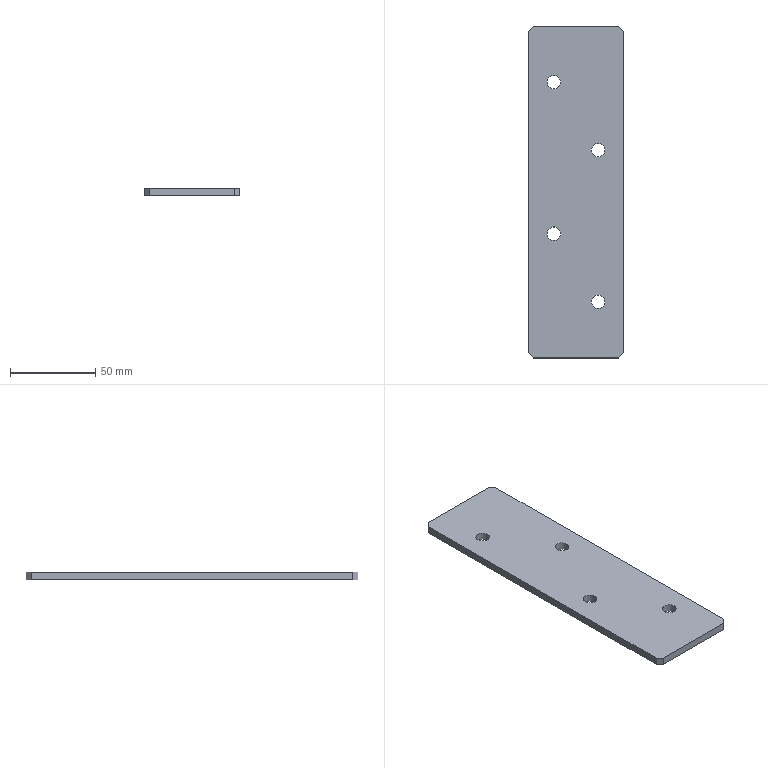Part | STEP file | 1_id70_x_t | 1 solid | 14 faces | box 56 x 195 x 4.5 mm | volume 48168 mm3 | plane 10 | cylinder 4 | commonest cylinder face diameters 7.938 x4
STEP:
#1=CARTESIAN_POINT('',(0.,0.,0.));
#2=DIRECTION('',(0.,0.,1.));
#3=DIRECTION('',(1.,0.,0.));
#4=AXIS2_PLACEMENT_3D('',#1,#2,#3);
#5=CARTESIAN_POINT('',(489.325,80.,86.035));
#6=VERTEX_POINT('',#5);
#7=CARTESIAN_POINT('',(489.325,80.,90.535));
#8=VERTEX_POINT('',#7);
#9=CARTESIAN_POINT('',(489.325,80.,86.035));
#10=DIRECTION('',(0.,0.,1.));
#11=VECTOR('',#10,1.);
#12=LINE('',#9,#11);
#13=CARTESIAN_POINT('',(489.325,80.,86.035));
#14=DIRECTION('',(0.7071,-0.7071,0.));
#15=DIRECTION('',(0.7071,0.7071,0.));
#16=AXIS2_PLACEMENT_3D('',#13,#14,#15);
#17=PLANE('',#16);
#18=CARTESIAN_POINT('',(0.,0.));
#19=DIRECTION('',(0.,1.));
#20=VECTOR('',#19,1.);
#21=LINE('',#18,#20);
#22=(GEOMETRIC_REPRESENTATION_CONTEXT(2)PARAMETRIC_REPRESENTATION_CONTEXT()REPRESENTATION_CONTEXT('',''));
#23=DEFINITIONAL_REPRESENTATION('',(#21),#22);
#24=PCURVE('',#17,#23);
#25=CARTESIAN_POINT('',(491.788,80.,86.035));
#26=DIRECTION('',(0.,-1.,0.));
#27=DIRECTION('',(1.,0.,0.));
#28=AXIS2_PLACEMENT_3D('',#25,#26,#27);
#29=PLANE('',#28);
#30=CARTESIAN_POINT('',(-2.463,0.));
#31=DIRECTION('',(0.,1.));
#32=VECTOR('',#31,1.);
#33=LINE('',#30,#32);
#34=(GEOMETRIC_REPRESENTATION_CONTEXT(2)PARAMETRIC_REPRESENTATION_CONTEXT()REPRESENTATION_CONTEXT('',''));
#35=DEFINITIONAL_REPRESENTATION('',(#33),#34);
#36=PCURVE('',#29,#35);
#37=SURFACE_CURVE('',#12,(#24,#36),.PCURVE_S1.);
#38=EDGE_CURVE('',#6,#8,#37,.T.);
#39=ORIENTED_EDGE('',*,*,#38,.F.);
#40=CARTESIAN_POINT('',(492.325,83.,86.035));
#41=VERTEX_POINT('',#40);
#42=CARTESIAN_POINT('',(489.325,80.,86.035));
#43=DIRECTION('',(0.7071,0.7071,0.));
#44=VECTOR('',#43,1.);
#45=LINE('',#42,#44);
#46=CARTESIAN_POINT('',(0.,0.));
#47=DIRECTION('',(1.,0.));
#48=VECTOR('',#47,1.);
#49=LINE('',#46,#48);
#50=(GEOMETRIC_REPRESENTATION_CONTEXT(2)PARAMETRIC_REPRESENTATION_CONTEXT()REPRESENTATION_CONTEXT('',''));
#51=DEFINITIONAL_REPRESENTATION('',(#49),#50);
#52=PCURVE('',#17,#51);
#53=CARTESIAN_POINT('',(491.788,255.,86.035));
#54=DIRECTION('',(0.,0.,1.));
#55=DIRECTION('',(1.,0.,0.));
#56=AXIS2_PLACEMENT_3D('',#53,#54,#55);
#57=PLANE('',#56);
#58=CARTESIAN_POINT('',(-2.463,-175.));
#59=DIRECTION('',(0.7071,0.7071));
#60=VECTOR('',#59,1.);
#61=LINE('',#58,#60);
#62=(GEOMETRIC_REPRESENTATION_CONTEXT(2)PARAMETRIC_REPRESENTATION_CONTEXT()REPRESENTATION_CONTEXT('',''));
#63=DEFINITIONAL_REPRESENTATION('',(#61),#62);
#64=PCURVE('',#57,#63);
#65=SURFACE_CURVE('',#45,(#52,#64),.PCURVE_S1.);
#66=EDGE_CURVE('',#6,#41,#65,.T.);
#67=ORIENTED_EDGE('',*,*,#66,.T.);
#68=CARTESIAN_POINT('',(492.325,83.,90.535));
#69=VERTEX_POINT('',#68);
#70=CARTESIAN_POINT('',(492.325,83.,86.035));
#71=DIRECTION('',(0.,0.,1.));
#72=VECTOR('',#71,1.);
#73=LINE('',#70,#72);
#74=CARTESIAN_POINT('',(4.243,0.));
#75=DIRECTION('',(0.,1.));
#76=VECTOR('',#75,1.);
#77=LINE('',#74,#76);
#78=(GEOMETRIC_REPRESENTATION_CONTEXT(2)PARAMETRIC_REPRESENTATION_CONTEXT()REPRESENTATION_CONTEXT('',''));
#79=DEFINITIONAL_REPRESENTATION('',(#77),#78);
#80=PCURVE('',#17,#79);
#81=CARTESIAN_POINT('',(492.325,255.,86.035));
#82=DIRECTION('',(1.,0.,0.));
#83=DIRECTION('',(0.,1.,0.));
#84=AXIS2_PLACEMENT_3D('',#81,#82,#83);
#85=PLANE('',#84);
#86=CARTESIAN_POINT('',(-172.,0.));
#87=DIRECTION('',(0.,1.));
#88=VECTOR('',#87,1.);
#89=LINE('',#86,#88);
#90=(GEOMETRIC_REPRESENTATION_CONTEXT(2)PARAMETRIC_REPRESENTATION_CONTEXT()REPRESENTATION_CONTEXT('',''));
#91=DEFINITIONAL_REPRESENTATION('',(#89),#90);
#92=PCURVE('',#85,#91);
#93=SURFACE_CURVE('',#73,(#80,#92),.PCURVE_S1.);
#94=EDGE_CURVE('',#41,#69,#93,.T.);
#95=ORIENTED_EDGE('',*,*,#94,.T.);
#96=CARTESIAN_POINT('',(489.325,80.,90.535));
#97=DIRECTION('',(0.7071,0.7071,0.));
#98=VECTOR('',#97,1.);
#99=LINE('',#96,#98);
#100=CARTESIAN_POINT('',(0.,4.5));
#101=DIRECTION('',(1.,0.));
#102=VECTOR('',#101,1.);
#103=LINE('',#100,#102);
#104=(GEOMETRIC_REPRESENTATION_CONTEXT(2)PARAMETRIC_REPRESENTATION_CONTEXT()REPRESENTATION_CONTEXT('',''));
#105=DEFINITIONAL_REPRESENTATION('',(#103),#104);
#106=PCURVE('',#17,#105);
#107=CARTESIAN_POINT('',(491.788,255.,90.535));
#108=DIRECTION('',(0.,0.,1.));
#109=DIRECTION('',(1.,0.,0.));
#110=AXIS2_PLACEMENT_3D('',#107,#108,#109);
#111=PLANE('',#110);
#112=CARTESIAN_POINT('',(-2.463,-175.));
#113=DIRECTION('',(0.7071,0.7071));
#114=VECTOR('',#113,1.);
#115=LINE('',#112,#114);
#116=(GEOMETRIC_REPRESENTATION_CONTEXT(2)PARAMETRIC_REPRESENTATION_CONTEXT()REPRESENTATION_CONTEXT('',''));
#117=DEFINITIONAL_REPRESENTATION('',(#115),#116);
#118=PCURVE('',#111,#117);
#119=SURFACE_CURVE('',#99,(#106,#118),.PCURVE_S1.);
#120=EDGE_CURVE('',#8,#69,#119,.T.);
#121=ORIENTED_EDGE('',*,*,#120,.F.);
#122=EDGE_LOOP('',(#39,#67,#95,#121));
#123=FACE_BOUND('',#122,.T.);
#124=ADVANCED_FACE('',(#123),#17,.T.);
#125=ORIENTED_EDGE('',*,*,#94,.F.);
#126=CARTESIAN_POINT('',(492.325,272.,86.035));
#127=VERTEX_POINT('',#126);
#128=CARTESIAN_POINT('',(492.325,255.,86.035));
#129=DIRECTION('',(0.,-1.,0.));
#130=VECTOR('',#129,1.);
#131=LINE('',#128,#130);
#132=CARTESIAN_POINT('',(0.,0.));
#133=DIRECTION('',(-1.,0.));
#134=VECTOR('',#133,1.);
#135=LINE('',#132,#134);
#136=(GEOMETRIC_REPRESENTATION_CONTEXT(2)PARAMETRIC_REPRESENTATION_CONTEXT()REPRESENTATION_CONTEXT('',''));
#137=DEFINITIONAL_REPRESENTATION('',(#135),#136);
#138=PCURVE('',#85,#137);
#139=CARTESIAN_POINT('',(0.5375,0.));
#140=DIRECTION('',(0.,-1.));
#141=VECTOR('',#140,1.);
#142=LINE('',#139,#141);
#143=(GEOMETRIC_REPRESENTATION_CONTEXT(2)PARAMETRIC_REPRESENTATION_CONTEXT()REPRESENTATION_CONTEXT('',''));
#144=DEFINITIONAL_REPRESENTATION('',(#142),#143);
#145=PCURVE('',#57,#144);
#146=SURFACE_CURVE('',#131,(#138,#145),.PCURVE_S1.);
#147=EDGE_CURVE('',#127,#41,#146,.T.);
#148=ORIENTED_EDGE('',*,*,#147,.F.);
#149=CARTESIAN_POINT('',(492.325,272.,90.535));
#150=VERTEX_POINT('',#149);
#151=CARTESIAN_POINT('',(492.325,272.,86.035));
#152=DIRECTION('',(0.,0.,1.));
#153=VECTOR('',#152,1.);
#154=LINE('',#151,#153);
#155=CARTESIAN_POINT('',(17.,0.));
#156=DIRECTION('',(0.,1.));
#157=VECTOR('',#156,1.);
#158=LINE('',#155,#157);
#159=(GEOMETRIC_REPRESENTATION_CONTEXT(2)PARAMETRIC_REPRESENTATION_CONTEXT()REPRESENTATION_CONTEXT('',''));
#160=DEFINITIONAL_REPRESENTATION('',(#158),#159);
#161=PCURVE('',#85,#160);
#162=CARTESIAN_POINT('',(492.325,272.,86.035));
#163=DIRECTION('',(0.7071,0.7071,0.));
#164=DIRECTION('',(-0.7071,0.7071,0.));
#165=AXIS2_PLACEMENT_3D('',#162,#163,#164);
#166=PLANE('',#165);
#167=CARTESIAN_POINT('',(0.,0.));
#168=DIRECTION('',(0.,1.));
#169=VECTOR('',#168,1.);
#170=LINE('',#167,#169);
#171=(GEOMETRIC_REPRESENTATION_CONTEXT(2)PARAMETRIC_REPRESENTATION_CONTEXT()REPRESENTATION_CONTEXT('',''));
#172=DEFINITIONAL_REPRESENTATION('',(#170),#171);
#173=PCURVE('',#166,#172);
#174=SURFACE_CURVE('',#154,(#161,#173),.PCURVE_S1.);
#175=EDGE_CURVE('',#127,#150,#174,.T.);
#176=ORIENTED_EDGE('',*,*,#175,.T.);
#177=CARTESIAN_POINT('',(492.325,255.,90.535));
#178=DIRECTION('',(0.,-1.,0.));
#179=VECTOR('',#178,1.);
#180=LINE('',#177,#179);
#181=CARTESIAN_POINT('',(0.,4.5));
#182=DIRECTION('',(-1.,0.));
#183=VECTOR('',#182,1.);
#184=LINE('',#181,#183);
#185=(GEOMETRIC_REPRESENTATION_CONTEXT(2)PARAMETRIC_REPRESENTATION_CONTEXT()REPRESENTATION_CONTEXT('',''));
#186=DEFINITIONAL_REPRESENTATION('',(#184),#185);
#187=PCURVE('',#85,#186);
#188=CARTESIAN_POINT('',(0.5375,0.));
#189=DIRECTION('',(0.,-1.));
#190=VECTOR('',#189,1.);
#191=LINE('',#188,#190);
#192=(GEOMETRIC_REPRESENTATION_CONTEXT(2)PARAMETRIC_REPRESENTATION_CONTEXT()REPRESENTATION_CONTEXT('',''));
#193=DEFINITIONAL_REPRESENTATION('',(#191),#192);
#194=PCURVE('',#111,#193);
#195=SURFACE_CURVE('',#180,(#187,#194),.PCURVE_S1.);
#196=EDGE_CURVE('',#150,#69,#195,.T.);
#197=ORIENTED_EDGE('',*,*,#196,.T.);
#198=EDGE_LOOP('',(#125,#148,#176,#197));
#199=FACE_BOUND('',#198,.T.);
#200=ADVANCED_FACE('',(#199),#85,.T.);
#201=ORIENTED_EDGE('',*,*,#175,.F.);
#202=CARTESIAN_POINT('',(489.325,275.,86.035));
#203=VERTEX_POINT('',#202);
#204=CARTESIAN_POINT('',(492.325,272.,86.035));
#205=DIRECTION('',(-0.7071,0.7071,0.));
#206=VECTOR('',#205,1.);
#207=LINE('',#204,#206);
#208=CARTESIAN_POINT('',(0.,0.));
#209=DIRECTION('',(1.,0.));
#210=VECTOR('',#209,1.);
#211=LINE('',#208,#210);
#212=(GEOMETRIC_REPRESENTATION_CONTEXT(2)PARAMETRIC_REPRESENTATION_CONTEXT()REPRESENTATION_CONTEXT('',''));
#213=DEFINITIONAL_REPRESENTATION('',(#211),#212);
#214=PCURVE('',#166,#213);
#215=CARTESIAN_POINT('',(0.5375,17.));
#216=DIRECTION('',(-0.7071,0.7071));
#217=VECTOR('',#216,1.);
#218=LINE('',#215,#217);
#219=(GEOMETRIC_REPRESENTATION_CONTEXT(2)PARAMETRIC_REPRESENTATION_CONTEXT()REPRESENTATION_CONTEXT('',''));
#220=DEFINITIONAL_REPRESENTATION('',(#218),#219);
#221=PCURVE('',#57,#220);
#222=SURFACE_CURVE('',#207,(#214,#221),.PCURVE_S1.);
#223=EDGE_CURVE('',#127,#203,#222,.T.);
#224=ORIENTED_EDGE('',*,*,#223,.T.);
#225=CARTESIAN_POINT('',(489.325,275.,90.535));
#226=VERTEX_POINT('',#225);
#227=CARTESIAN_POINT('',(489.325,275.,86.035));
#228=DIRECTION('',(0.,0.,1.));
#229=VECTOR('',#228,1.);
#230=LINE('',#227,#229);
#231=CARTESIAN_POINT('',(4.243,0.));
#232=DIRECTION('',(0.,1.));
#233=VECTOR('',#232,1.);
#234=LINE('',#231,#233);
#235=(GEOMETRIC_REPRESENTATION_CONTEXT(2)PARAMETRIC_REPRESENTATION_CONTEXT()REPRESENTATION_CONTEXT('',''));
#236=DEFINITIONAL_REPRESENTATION('',(#234),#235);
#237=PCURVE('',#166,#236);
#238=CARTESIAN_POINT('',(491.788,275.,86.035));
#239=DIRECTION('',(0.,-1.,0.));
#240=DIRECTION('',(1.,0.,0.));
#241=AXIS2_PLACEMENT_3D('',#238,#239,#240);
#242=PLANE('',#241);
#243=CARTESIAN_POINT('',(-2.463,0.));
#244=DIRECTION('',(0.,1.));
#245=VECTOR('',#244,1.);
#246=LINE('',#243,#245);
#247=(GEOMETRIC_REPRESENTATION_CONTEXT(2)PARAMETRIC_REPRESENTATION_CONTEXT()REPRESENTATION_CONTEXT('',''));
#248=DEFINITIONAL_REPRESENTATION('',(#246),#247);
#249=PCURVE('',#242,#248);
#250=SURFACE_CURVE('',#230,(#237,#249),.PCURVE_S1.);
#251=EDGE_CURVE('',#203,#226,#250,.T.);
#252=ORIENTED_EDGE('',*,*,#251,.T.);
#253=CARTESIAN_POINT('',(492.325,272.,90.535));
#254=DIRECTION('',(-0.7071,0.7071,0.));
#255=VECTOR('',#254,1.);
#256=LINE('',#253,#255);
#257=CARTESIAN_POINT('',(0.,4.5));
#258=DIRECTION('',(1.,0.));
#259=VECTOR('',#258,1.);
#260=LINE('',#257,#259);
#261=(GEOMETRIC_REPRESENTATION_CONTEXT(2)PARAMETRIC_REPRESENTATION_CONTEXT()REPRESENTATION_CONTEXT('',''));
#262=DEFINITIONAL_REPRESENTATION('',(#260),#261);
#263=PCURVE('',#166,#262);
#264=CARTESIAN_POINT('',(0.5375,17.));
#265=DIRECTION('',(-0.7071,0.7071));
#266=VECTOR('',#265,1.);
#267=LINE('',#264,#266);
#268=(GEOMETRIC_REPRESENTATION_CONTEXT(2)PARAMETRIC_REPRESENTATION_CONTEXT()REPRESENTATION_CONTEXT('',''));
#269=DEFINITIONAL_REPRESENTATION('',(#267),#268);
#270=PCURVE('',#111,#269);
#271=SURFACE_CURVE('',#256,(#263,#270),.PCURVE_S1.);
#272=EDGE_CURVE('',#150,#226,#271,.T.);
#273=ORIENTED_EDGE('',*,*,#272,.F.);
#274=EDGE_LOOP('',(#201,#224,#252,#273));
#275=FACE_BOUND('',#274,.T.);
#276=ADVANCED_FACE('',(#275),#166,.T.);
#277=ORIENTED_EDGE('',*,*,#251,.F.);
#278=CARTESIAN_POINT('',(439.325,275.,86.035));
#279=VERTEX_POINT('',#278);
#280=CARTESIAN_POINT('',(491.788,275.,86.035));
#281=DIRECTION('',(-1.,0.,0.));
#282=VECTOR('',#281,1.);
#283=LINE('',#280,#282);
#284=CARTESIAN_POINT('',(0.,0.));
#285=DIRECTION('',(-1.,0.));
#286=VECTOR('',#285,1.);
#287=LINE('',#284,#286);
#288=(GEOMETRIC_REPRESENTATION_CONTEXT(2)PARAMETRIC_REPRESENTATION_CONTEXT()REPRESENTATION_CONTEXT('',''));
#289=DEFINITIONAL_REPRESENTATION('',(#287),#288);
#290=PCURVE('',#242,#289);
#291=CARTESIAN_POINT('',(0.,20.));
#292=DIRECTION('',(-1.,0.));
#293=VECTOR('',#292,1.);
#294=LINE('',#291,#293);
#295=(GEOMETRIC_REPRESENTATION_CONTEXT(2)PARAMETRIC_REPRESENTATION_CONTEXT()REPRESENTATION_CONTEXT('',''));
#296=DEFINITIONAL_REPRESENTATION('',(#294),#295);
#297=PCURVE('',#57,#296);
#298=SURFACE_CURVE('',#283,(#290,#297),.PCURVE_S1.);
#299=EDGE_CURVE('',#203,#279,#298,.T.);
#300=ORIENTED_EDGE('',*,*,#299,.T.);
#301=CARTESIAN_POINT('',(439.325,275.,90.535));
#302=VERTEX_POINT('',#301);
#303=CARTESIAN_POINT('',(439.325,275.,86.035));
#304=DIRECTION('',(0.,0.,1.));
#305=VECTOR('',#304,1.);
#306=LINE('',#303,#305);
#307=CARTESIAN_POINT('',(-52.463,0.));
#308=DIRECTION('',(0.,1.));
#309=VECTOR('',#308,1.);
#310=LINE('',#307,#309);
#311=(GEOMETRIC_REPRESENTATION_CONTEXT(2)PARAMETRIC_REPRESENTATION_CONTEXT()REPRESENTATION_CONTEXT('',''));
#312=DEFINITIONAL_REPRESENTATION('',(#310),#311);
#313=PCURVE('',#242,#312);
#314=CARTESIAN_POINT('',(439.325,275.,86.035));
#315=DIRECTION('',(-0.7071,0.7071,0.));
#316=DIRECTION('',(-0.7071,-0.7071,0.));
#317=AXIS2_PLACEMENT_3D('',#314,#315,#316);
#318=PLANE('',#317);
#319=CARTESIAN_POINT('',(0.,0.));
#320=DIRECTION('',(0.,1.));
#321=VECTOR('',#320,1.);
#322=LINE('',#319,#321);
#323=(GEOMETRIC_REPRESENTATION_CONTEXT(2)PARAMETRIC_REPRESENTATION_CONTEXT()REPRESENTATION_CONTEXT('',''));
#324=DEFINITIONAL_REPRESENTATION('',(#322),#323);
#325=PCURVE('',#318,#324);
#326=SURFACE_CURVE('',#306,(#313,#325),.PCURVE_S1.);
#327=EDGE_CURVE('',#279,#302,#326,.T.);
#328=ORIENTED_EDGE('',*,*,#327,.T.);
#329=CARTESIAN_POINT('',(491.788,275.,90.535));
#330=DIRECTION('',(-1.,0.,0.));
#331=VECTOR('',#330,1.);
#332=LINE('',#329,#331);
#333=CARTESIAN_POINT('',(0.,4.5));
#334=DIRECTION('',(-1.,0.));
#335=VECTOR('',#334,1.);
#336=LINE('',#333,#335);
#337=(GEOMETRIC_REPRESENTATION_CONTEXT(2)PARAMETRIC_REPRESENTATION_CONTEXT()REPRESENTATION_CONTEXT('',''));
#338=DEFINITIONAL_REPRESENTATION('',(#336),#337);
#339=PCURVE('',#242,#338);
#340=CARTESIAN_POINT('',(0.,20.));
#341=DIRECTION('',(-1.,0.));
#342=VECTOR('',#341,1.);
#343=LINE('',#340,#342);
#344=(GEOMETRIC_REPRESENTATION_CONTEXT(2)PARAMETRIC_REPRESENTATION_CONTEXT()REPRESENTATION_CONTEXT('',''));
#345=DEFINITIONAL_REPRESENTATION('',(#343),#344);
#346=PCURVE('',#111,#345);
#347=SURFACE_CURVE('',#332,(#339,#346),.PCURVE_S1.);
#348=EDGE_CURVE('',#226,#302,#347,.T.);
#349=ORIENTED_EDGE('',*,*,#348,.F.);
#350=EDGE_LOOP('',(#277,#300,#328,#349));
#351=FACE_BOUND('',#350,.T.);
#352=ADVANCED_FACE('',(#351),#242,.F.);
#353=ORIENTED_EDGE('',*,*,#327,.F.);
#354=CARTESIAN_POINT('',(436.325,272.,86.035));
#355=VERTEX_POINT('',#354);
#356=CARTESIAN_POINT('',(439.325,275.,86.035));
#357=DIRECTION('',(-0.7071,-0.7071,0.));
#358=VECTOR('',#357,1.);
#359=LINE('',#356,#358);
#360=CARTESIAN_POINT('',(0.,0.));
#361=DIRECTION('',(1.,0.));
#362=VECTOR('',#361,1.);
#363=LINE('',#360,#362);
#364=(GEOMETRIC_REPRESENTATION_CONTEXT(2)PARAMETRIC_REPRESENTATION_CONTEXT()REPRESENTATION_CONTEXT('',''));
#365=DEFINITIONAL_REPRESENTATION('',(#363),#364);
#366=PCURVE('',#318,#365);
#367=CARTESIAN_POINT('',(-52.463,20.));
#368=DIRECTION('',(-0.7071,-0.7071));
#369=VECTOR('',#368,1.);
#370=LINE('',#367,#369);
#371=(GEOMETRIC_REPRESENTATION_CONTEXT(2)PARAMETRIC_REPRESENTATION_CONTEXT()REPRESENTATION_CONTEXT('',''));
#372=DEFINITIONAL_REPRESENTATION('',(#370),#371);
#373=PCURVE('',#57,#372);
#374=SURFACE_CURVE('',#359,(#366,#373),.PCURVE_S1.);
#375=EDGE_CURVE('',#279,#355,#374,.T.);
#376=ORIENTED_EDGE('',*,*,#375,.T.);
#377=CARTESIAN_POINT('',(436.325,272.,90.535));
#378=VERTEX_POINT('',#377);
#379=CARTESIAN_POINT('',(436.325,272.,86.035));
#380=DIRECTION('',(0.,0.,1.));
#381=VECTOR('',#380,1.);
#382=LINE('',#379,#381);
#383=CARTESIAN_POINT('',(4.243,0.));
#384=DIRECTION('',(0.,1.));
#385=VECTOR('',#384,1.);
#386=LINE('',#383,#385);
#387=(GEOMETRIC_REPRESENTATION_CONTEXT(2)PARAMETRIC_REPRESENTATION_CONTEXT()REPRESENTATION_CONTEXT('',''));
#388=DEFINITIONAL_REPRESENTATION('',(#386),#387);
#389=PCURVE('',#318,#388);
#390=CARTESIAN_POINT('',(436.325,255.,86.035));
#391=DIRECTION('',(1.,0.,0.));
#392=DIRECTION('',(0.,1.,0.));
#393=AXIS2_PLACEMENT_3D('',#390,#391,#392);
#394=PLANE('',#393);
#395=CARTESIAN_POINT('',(17.,0.));
#396=DIRECTION('',(0.,1.));
#397=VECTOR('',#396,1.);
#398=LINE('',#395,#397);
#399=(GEOMETRIC_REPRESENTATION_CONTEXT(2)PARAMETRIC_REPRESENTATION_CONTEXT()REPRESENTATION_CONTEXT('',''));
#400=DEFINITIONAL_REPRESENTATION('',(#398),#399);
#401=PCURVE('',#394,#400);
#402=SURFACE_CURVE('',#382,(#389,#401),.PCURVE_S1.);
#403=EDGE_CURVE('',#355,#378,#402,.T.);
#404=ORIENTED_EDGE('',*,*,#403,.T.);
#405=CARTESIAN_POINT('',(439.325,275.,90.535));
#406=DIRECTION('',(-0.7071,-0.7071,0.));
#407=VECTOR('',#406,1.);
#408=LINE('',#405,#407);
#409=CARTESIAN_POINT('',(0.,4.5));
#410=DIRECTION('',(1.,0.));
#411=VECTOR('',#410,1.);
#412=LINE('',#409,#411);
#413=(GEOMETRIC_REPRESENTATION_CONTEXT(2)PARAMETRIC_REPRESENTATION_CONTEXT()REPRESENTATION_CONTEXT('',''));
#414=DEFINITIONAL_REPRESENTATION('',(#412),#413);
#415=PCURVE('',#318,#414);
#416=CARTESIAN_POINT('',(-52.463,20.));
#417=DIRECTION('',(-0.7071,-0.7071));
#418=VECTOR('',#417,1.);
#419=LINE('',#416,#418);
#420=(GEOMETRIC_REPRESENTATION_CONTEXT(2)PARAMETRIC_REPRESENTATION_CONTEXT()REPRESENTATION_CONTEXT('',''));
#421=DEFINITIONAL_REPRESENTATION('',(#419),#420);
#422=PCURVE('',#111,#421);
#423=SURFACE_CURVE('',#408,(#415,#422),.PCURVE_S1.);
#424=EDGE_CURVE('',#302,#378,#423,.T.);
#425=ORIENTED_EDGE('',*,*,#424,.F.);
#426=EDGE_LOOP('',(#353,#376,#404,#425));
#427=FACE_BOUND('',#426,.T.);
#428=ADVANCED_FACE('',(#427),#318,.T.);
#429=ORIENTED_EDGE('',*,*,#403,.F.);
#430=CARTESIAN_POINT('',(436.325,83.,86.035));
#431=VERTEX_POINT('',#430);
#432=CARTESIAN_POINT('',(436.325,255.,86.035));
#433=DIRECTION('',(0.,1.,0.));
#434=VECTOR('',#433,1.);
#435=LINE('',#432,#434);
#436=CARTESIAN_POINT('',(0.,0.));
#437=DIRECTION('',(1.,0.));
#438=VECTOR('',#437,1.);
#439=LINE('',#436,#438);
#440=(GEOMETRIC_REPRESENTATION_CONTEXT(2)PARAMETRIC_REPRESENTATION_CONTEXT()REPRESENTATION_CONTEXT('',''));
#441=DEFINITIONAL_REPRESENTATION('',(#439),#440);
#442=PCURVE('',#394,#441);
#443=CARTESIAN_POINT('',(-55.463,0.));
#444=DIRECTION('',(0.,1.));
#445=VECTOR('',#444,1.);
#446=LINE('',#443,#445);
#447=(GEOMETRIC_REPRESENTATION_CONTEXT(2)PARAMETRIC_REPRESENTATION_CONTEXT()REPRESENTATION_CONTEXT('',''));
#448=DEFINITIONAL_REPRESENTATION('',(#446),#447);
#449=PCURVE('',#57,#448);
#450=SURFACE_CURVE('',#435,(#442,#449),.PCURVE_S1.);
#451=EDGE_CURVE('',#431,#355,#450,.T.);
#452=ORIENTED_EDGE('',*,*,#451,.F.);
#453=CARTESIAN_POINT('',(436.325,83.,90.535));
#454=VERTEX_POINT('',#453);
#455=CARTESIAN_POINT('',(436.325,83.,86.035));
#456=DIRECTION('',(0.,0.,1.));
#457=VECTOR('',#456,1.);
#458=LINE('',#455,#457);
#459=CARTESIAN_POINT('',(-172.,0.));
#460=DIRECTION('',(0.,1.));
#461=VECTOR('',#460,1.);
#462=LINE('',#459,#461);
#463=(GEOMETRIC_REPRESENTATION_CONTEXT(2)PARAMETRIC_REPRESENTATION_CONTEXT()REPRESENTATION_CONTEXT('',''));
#464=DEFINITIONAL_REPRESENTATION('',(#462),#463);
#465=PCURVE('',#394,#464);
#466=CARTESIAN_POINT('',(436.325,83.,86.035));
#467=DIRECTION('',(-0.7071,-0.7071,0.));
#468=DIRECTION('',(0.7071,-0.7071,0.));
#469=AXIS2_PLACEMENT_3D('',#466,#467,#468);
#470=PLANE('',#469);
#471=CARTESIAN_POINT('',(0.,0.));
#472=DIRECTION('',(0.,1.));
#473=VECTOR('',#472,1.);
#474=LINE('',#471,#473);
#475=(GEOMETRIC_REPRESENTATION_CONTEXT(2)PARAMETRIC_REPRESENTATION_CONTEXT()REPRESENTATION_CONTEXT('',''));
#476=DEFINITIONAL_REPRESENTATION('',(#474),#475);
#477=PCURVE('',#470,#476);
#478=SURFACE_CURVE('',#458,(#465,#477),.PCURVE_S1.);
#479=EDGE_CURVE('',#431,#454,#478,.T.);
#480=ORIENTED_EDGE('',*,*,#479,.T.);
#481=CARTESIAN_POINT('',(436.325,255.,90.535));
#482=DIRECTION('',(0.,1.,0.));
#483=VECTOR('',#482,1.);
#484=LINE('',#481,#483);
#485=CARTESIAN_POINT('',(0.,4.5));
#486=DIRECTION('',(1.,0.));
#487=VECTOR('',#486,1.);
#488=LINE('',#485,#487);
#489=(GEOMETRIC_REPRESENTATION_CONTEXT(2)PARAMETRIC_REPRESENTATION_CONTEXT()REPRESENTATION_CONTEXT('',''));
#490=DEFINITIONAL_REPRESENTATION('',(#488),#489);
#491=PCURVE('',#394,#490);
#492=CARTESIAN_POINT('',(-55.463,0.));
#493=DIRECTION('',(0.,1.));
#494=VECTOR('',#493,1.);
#495=LINE('',#492,#494);
#496=(GEOMETRIC_REPRESENTATION_CONTEXT(2)PARAMETRIC_REPRESENTATION_CONTEXT()REPRESENTATION_CONTEXT('',''));
#497=DEFINITIONAL_REPRESENTATION('',(#495),#496);
#498=PCURVE('',#111,#497);
#499=SURFACE_CURVE('',#484,(#491,#498),.PCURVE_S1.);
#500=EDGE_CURVE('',#454,#378,#499,.T.);
#501=ORIENTED_EDGE('',*,*,#500,.T.);
#502=EDGE_LOOP('',(#429,#452,#480,#501));
#503=FACE_BOUND('',#502,.T.);
#504=ADVANCED_FACE('',(#503),#394,.F.);
#505=ORIENTED_EDGE('',*,*,#479,.F.);
#506=CARTESIAN_POINT('',(439.325,80.,86.035));
#507=VERTEX_POINT('',#506);
#508=CARTESIAN_POINT('',(436.325,83.,86.035));
#509=DIRECTION('',(0.7071,-0.7071,0.));
#510=VECTOR('',#509,1.);
#511=LINE('',#508,#510);
#512=CARTESIAN_POINT('',(0.,0.));
#513=DIRECTION('',(1.,0.));
#514=VECTOR('',#513,1.);
#515=LINE('',#512,#514);
#516=(GEOMETRIC_REPRESENTATION_CONTEXT(2)PARAMETRIC_REPRESENTATION_CONTEXT()REPRESENTATION_CONTEXT('',''));
#517=DEFINITIONAL_REPRESENTATION('',(#515),#516);
#518=PCURVE('',#470,#517);
#519=CARTESIAN_POINT('',(-55.463,-172.));
#520=DIRECTION('',(0.7071,-0.7071));
#521=VECTOR('',#520,1.);
#522=LINE('',#519,#521);
#523=(GEOMETRIC_REPRESENTATION_CONTEXT(2)PARAMETRIC_REPRESENTATION_CONTEXT()REPRESENTATION_CONTEXT('',''));
#524=DEFINITIONAL_REPRESENTATION('',(#522),#523);
#525=PCURVE('',#57,#524);
#526=SURFACE_CURVE('',#511,(#518,#525),.PCURVE_S1.);
#527=EDGE_CURVE('',#431,#507,#526,.T.);
#528=ORIENTED_EDGE('',*,*,#527,.T.);
#529=CARTESIAN_POINT('',(439.325,80.,90.535));
#530=VERTEX_POINT('',#529);
#531=CARTESIAN_POINT('',(439.325,80.,86.035));
#532=DIRECTION('',(0.,0.,1.));
#533=VECTOR('',#532,1.);
#534=LINE('',#531,#533);
#535=CARTESIAN_POINT('',(4.243,0.));
#536=DIRECTION('',(0.,1.));
#537=VECTOR('',#536,1.);
#538=LINE('',#535,#537);
#539=(GEOMETRIC_REPRESENTATION_CONTEXT(2)PARAMETRIC_REPRESENTATION_CONTEXT()REPRESENTATION_CONTEXT('',''));
#540=DEFINITIONAL_REPRESENTATION('',(#538),#539);
#541=PCURVE('',#470,#540);
#542=CARTESIAN_POINT('',(-52.463,0.));
#543=DIRECTION('',(0.,1.));
#544=VECTOR('',#543,1.);
#545=LINE('',#542,#544);
#546=(GEOMETRIC_REPRESENTATION_CONTEXT(2)PARAMETRIC_REPRESENTATION_CONTEXT()REPRESENTATION_CONTEXT('',''));
#547=DEFINITIONAL_REPRESENTATION('',(#545),#546);
#548=PCURVE('',#29,#547);
#549=SURFACE_CURVE('',#534,(#541,#548),.PCURVE_S1.);
#550=EDGE_CURVE('',#507,#530,#549,.T.);
#551=ORIENTED_EDGE('',*,*,#550,.T.);
#552=CARTESIAN_POINT('',(436.325,83.,90.535));
#553=DIRECTION('',(0.7071,-0.7071,0.));
#554=VECTOR('',#553,1.);
#555=LINE('',#552,#554);
#556=CARTESIAN_POINT('',(0.,4.5));
#557=DIRECTION('',(1.,0.));
#558=VECTOR('',#557,1.);
#559=LINE('',#556,#558);
#560=(GEOMETRIC_REPRESENTATION_CONTEXT(2)PARAMETRIC_REPRESENTATION_CONTEXT()REPRESENTATION_CONTEXT('',''));
#561=DEFINITIONAL_REPRESENTATION('',(#559),#560);
#562=PCURVE('',#470,#561);
#563=CARTESIAN_POINT('',(-55.463,-172.));
#564=DIRECTION('',(0.7071,-0.7071));
#565=VECTOR('',#564,1.);
#566=LINE('',#563,#565);
#567=(GEOMETRIC_REPRESENTATION_CONTEXT(2)PARAMETRIC_REPRESENTATION_CONTEXT()REPRESENTATION_CONTEXT('',''));
#568=DEFINITIONAL_REPRESENTATION('',(#566),#567);
#569=PCURVE('',#111,#568);
#570=SURFACE_CURVE('',#555,(#562,#569),.PCURVE_S1.);
#571=EDGE_CURVE('',#454,#530,#570,.T.);
#572=ORIENTED_EDGE('',*,*,#571,.F.);
#573=EDGE_LOOP('',(#505,#528,#551,#572));
#574=FACE_BOUND('',#573,.T.);
#575=ADVANCED_FACE('',(#574),#470,.T.);
#576=CARTESIAN_POINT('',(491.788,80.,86.035));
#577=DIRECTION('',(-1.,0.,0.));
#578=VECTOR('',#577,1.);
#579=LINE('',#576,#578);
#580=CARTESIAN_POINT('',(0.,0.));
#581=DIRECTION('',(-1.,0.));
#582=VECTOR('',#581,1.);
#583=LINE('',#580,#582);
#584=(GEOMETRIC_REPRESENTATION_CONTEXT(2)PARAMETRIC_REPRESENTATION_CONTEXT()REPRESENTATION_CONTEXT('',''));
#585=DEFINITIONAL_REPRESENTATION('',(#583),#584);
#586=PCURVE('',#29,#585);
#587=CARTESIAN_POINT('',(0.,-175.));
#588=DIRECTION('',(-1.,0.));
#589=VECTOR('',#588,1.);
#590=LINE('',#587,#589);
#591=(GEOMETRIC_REPRESENTATION_CONTEXT(2)PARAMETRIC_REPRESENTATION_CONTEXT()REPRESENTATION_CONTEXT('',''));
#592=DEFINITIONAL_REPRESENTATION('',(#590),#591);
#593=PCURVE('',#57,#592);
#594=SURFACE_CURVE('',#579,(#586,#593),.PCURVE_S1.);
#595=EDGE_CURVE('',#6,#507,#594,.T.);
#596=ORIENTED_EDGE('',*,*,#595,.F.);
#597=ORIENTED_EDGE('',*,*,#38,.T.);
#598=CARTESIAN_POINT('',(491.788,80.,90.535));
#599=DIRECTION('',(-1.,0.,0.));
#600=VECTOR('',#599,1.);
#601=LINE('',#598,#600);
#602=CARTESIAN_POINT('',(0.,4.5));
#603=DIRECTION('',(-1.,0.));
#604=VECTOR('',#603,1.);
#605=LINE('',#602,#604);
#606=(GEOMETRIC_REPRESENTATION_CONTEXT(2)PARAMETRIC_REPRESENTATION_CONTEXT()REPRESENTATION_CONTEXT('',''));
#607=DEFINITIONAL_REPRESENTATION('',(#605),#606);
#608=PCURVE('',#29,#607);
#609=CARTESIAN_POINT('',(0.,-175.));
#610=DIRECTION('',(-1.,0.));
#611=VECTOR('',#610,1.);
#612=LINE('',#609,#611);
#613=(GEOMETRIC_REPRESENTATION_CONTEXT(2)PARAMETRIC_REPRESENTATION_CONTEXT()REPRESENTATION_CONTEXT('',''));
#614=DEFINITIONAL_REPRESENTATION('',(#612),#613);
#615=PCURVE('',#111,#614);
#616=SURFACE_CURVE('',#601,(#608,#615),.PCURVE_S1.);
#617=EDGE_CURVE('',#8,#530,#616,.T.);
#618=ORIENTED_EDGE('',*,*,#617,.T.);
#619=ORIENTED_EDGE('',*,*,#550,.F.);
#620=EDGE_LOOP('',(#596,#597,#618,#619));
#621=FACE_BOUND('',#620,.T.);
#622=ADVANCED_FACE('',(#621),#29,.T.);
#623=CARTESIAN_POINT('',(455.294,242.,90.535));
#624=VERTEX_POINT('',#623);
#625=CARTESIAN_POINT('',(451.325,242.,90.535));
#626=DIRECTION('',(0.,0.,-1.));
#627=DIRECTION('',(1.,0.,0.));
#628=AXIS2_PLACEMENT_3D('',#625,#626,#627);
#629=CIRCLE('',#628,3.969);
#630=CARTESIAN_POINT('',(451.325,242.,86.035));
#631=DIRECTION('',(0.,0.,1.));
#632=DIRECTION('',(1.,0.,0.));
#633=AXIS2_PLACEMENT_3D('',#630,#631,#632);
#634=CYLINDRICAL_SURFACE('',#633,3.969);
#635=CARTESIAN_POINT('',(6.283,4.5));
#636=DIRECTION('',(-1.,0.));
#637=VECTOR('',#636,1.);
#638=LINE('',#635,#637);
#639=(GEOMETRIC_REPRESENTATION_CONTEXT(2)PARAMETRIC_REPRESENTATION_CONTEXT()REPRESENTATION_CONTEXT('',''));
#640=DEFINITIONAL_REPRESENTATION('',(#638),#639);
#641=PCURVE('',#634,#640);
#642=CARTESIAN_POINT('',(-36.494,-13.));
#643=CARTESIAN_POINT('',(-36.494,-19.874));
#644=CARTESIAN_POINT('',(-42.447,-16.437));
#645=CARTESIAN_POINT('',(-48.4,-13.));
#646=CARTESIAN_POINT('',(-42.447,-9.563));
#647=CARTESIAN_POINT('',(-36.494,-6.126));
#648=CARTESIAN_POINT('',(-36.494,-13.));
#649=(BOUNDED_CURVE()B_SPLINE_CURVE(2,(#642,#643,#644,#645,#646,#647,#648),.UNSPECIFIED.,.T.,.F.)B_SPLINE_CURVE_WITH_KNOTS((1,2,2,2,2,1),(-2.094,0.,2.094,4.189,6.283,8.378),.UNSPECIFIED.)CURVE()GEOMETRIC_REPRESENTATION_ITEM()RATIONAL_B_SPLINE_CURVE((1.,0.5,1.,0.5,1.,0.5,1.))REPRESENTATION_ITEM(''));
#650=(GEOMETRIC_REPRESENTATION_CONTEXT(2)PARAMETRIC_REPRESENTATION_CONTEXT()REPRESENTATION_CONTEXT('',''));
#651=DEFINITIONAL_REPRESENTATION('',(#649),#650);
#652=PCURVE('',#111,#651);
#653=SURFACE_CURVE('',#629,(#641,#652),.PCURVE_S1.);
#654=EDGE_CURVE('',#624,#624,#653,.T.);
#655=ORIENTED_EDGE('',*,*,#654,.T.);
#656=CARTESIAN_POINT('',(455.294,242.,86.035));
#657=VERTEX_POINT('',#656);
#658=CARTESIAN_POINT('',(455.294,242.,86.035));
#659=CARTESIAN_POINT('',(455.294,242.,90.535));
#660=B_SPLINE_CURVE_WITH_KNOTS('',1,(#658,#659),.UNSPECIFIED.,.F.,.F.,(2,2),(0.,4.5),.PIECEWISE_BEZIER_KNOTS.);
#661=CARTESIAN_POINT('',(0.,0.));
#662=DIRECTION('',(0.,1.));
#663=VECTOR('',#662,1.);
#664=LINE('',#661,#663);
#665=(GEOMETRIC_REPRESENTATION_CONTEXT(2)PARAMETRIC_REPRESENTATION_CONTEXT()REPRESENTATION_CONTEXT('',''));
#666=DEFINITIONAL_REPRESENTATION('',(#664),#665);
#667=PCURVE('',#634,#666);
#668=CARTESIAN_POINT('',(6.283,0.));
#669=DIRECTION('',(0.,1.));
#670=VECTOR('',#669,1.);
#671=LINE('',#668,#670);
#672=(GEOMETRIC_REPRESENTATION_CONTEXT(2)PARAMETRIC_REPRESENTATION_CONTEXT()REPRESENTATION_CONTEXT('',''));
#673=DEFINITIONAL_REPRESENTATION('',(#671),#672);
#674=PCURVE('',#634,#673);
#675=SEAM_CURVE('',#660,(#667,#674),.PCURVE_S1.);
#676=EDGE_CURVE('',#657,#624,#675,.T.);
#677=ORIENTED_EDGE('',*,*,#676,.F.);
#678=CARTESIAN_POINT('',(451.325,242.,86.035));
#679=DIRECTION('',(0.,0.,-1.));
#680=DIRECTION('',(1.,0.,0.));
#681=AXIS2_PLACEMENT_3D('',#678,#679,#680);
#682=CIRCLE('',#681,3.969);
#683=CARTESIAN_POINT('',(6.283,0.));
#684=DIRECTION('',(-1.,0.));
#685=VECTOR('',#684,1.);
#686=LINE('',#683,#685);
#687=(GEOMETRIC_REPRESENTATION_CONTEXT(2)PARAMETRIC_REPRESENTATION_CONTEXT()REPRESENTATION_CONTEXT('',''));
#688=DEFINITIONAL_REPRESENTATION('',(#686),#687);
#689=PCURVE('',#634,#688);
#690=CARTESIAN_POINT('',(-36.494,-13.));
#691=CARTESIAN_POINT('',(-36.494,-19.874));
#692=CARTESIAN_POINT('',(-42.447,-16.437));
#693=CARTESIAN_POINT('',(-48.4,-13.));
#694=CARTESIAN_POINT('',(-42.447,-9.563));
#695=CARTESIAN_POINT('',(-36.494,-6.126));
#696=CARTESIAN_POINT('',(-36.494,-13.));
#697=(BOUNDED_CURVE()B_SPLINE_CURVE(2,(#690,#691,#692,#693,#694,#695,#696),.UNSPECIFIED.,.T.,.F.)B_SPLINE_CURVE_WITH_KNOTS((1,2,2,2,2,1),(-2.094,0.,2.094,4.189,6.283,8.378),.UNSPECIFIED.)CURVE()GEOMETRIC_REPRESENTATION_ITEM()RATIONAL_B_SPLINE_CURVE((1.,0.5,1.,0.5,1.,0.5,1.))REPRESENTATION_ITEM(''));
#698=(GEOMETRIC_REPRESENTATION_CONTEXT(2)PARAMETRIC_REPRESENTATION_CONTEXT()REPRESENTATION_CONTEXT('',''));
#699=DEFINITIONAL_REPRESENTATION('',(#697),#698);
#700=PCURVE('',#57,#699);
#701=SURFACE_CURVE('',#682,(#689,#700),.PCURVE_S1.);
#702=EDGE_CURVE('',#657,#657,#701,.T.);
#703=ORIENTED_EDGE('',*,*,#702,.F.);
#704=ORIENTED_EDGE('',*,*,#676,.T.);
#705=EDGE_LOOP('',(#655,#677,#703,#704));
#706=FACE_BOUND('',#705,.F.);
#707=ADVANCED_FACE('',(#706),#634,.F.);
#708=CARTESIAN_POINT('',(481.294,202.,90.535));
#709=VERTEX_POINT('',#708);
#710=CARTESIAN_POINT('',(477.325,202.,90.535));
#711=DIRECTION('',(0.,0.,-1.));
#712=DIRECTION('',(1.,0.,0.));
#713=AXIS2_PLACEMENT_3D('',#710,#711,#712);
#714=CIRCLE('',#713,3.969);
#715=CARTESIAN_POINT('',(477.325,202.,86.035));
#716=DIRECTION('',(0.,0.,1.));
#717=DIRECTION('',(1.,0.,0.));
#718=AXIS2_PLACEMENT_3D('',#715,#716,#717);
#719=CYLINDRICAL_SURFACE('',#718,3.969);
#720=CARTESIAN_POINT('',(6.283,4.5));
#721=DIRECTION('',(-1.,0.));
#722=VECTOR('',#721,1.);
#723=LINE('',#720,#722);
#724=(GEOMETRIC_REPRESENTATION_CONTEXT(2)PARAMETRIC_REPRESENTATION_CONTEXT()REPRESENTATION_CONTEXT('',''));
#725=DEFINITIONAL_REPRESENTATION('',(#723),#724);
#726=PCURVE('',#719,#725);
#727=CARTESIAN_POINT('',(-10.494,-53.));
#728=CARTESIAN_POINT('',(-10.494,-59.874));
#729=CARTESIAN_POINT('',(-16.447,-56.437));
#730=CARTESIAN_POINT('',(-22.4,-53.));
#731=CARTESIAN_POINT('',(-16.447,-49.563));
#732=CARTESIAN_POINT('',(-10.494,-46.126));
#733=CARTESIAN_POINT('',(-10.494,-53.));
#734=(BOUNDED_CURVE()B_SPLINE_CURVE(2,(#727,#728,#729,#730,#731,#732,#733),.UNSPECIFIED.,.T.,.F.)B_SPLINE_CURVE_WITH_KNOTS((1,2,2,2,2,1),(-2.094,0.,2.094,4.189,6.283,8.378),.UNSPECIFIED.)CURVE()GEOMETRIC_REPRESENTATION_ITEM()RATIONAL_B_SPLINE_CURVE((1.,0.5,1.,0.5,1.,0.5,1.))REPRESENTATION_ITEM(''));
#735=(GEOMETRIC_REPRESENTATION_CONTEXT(2)PARAMETRIC_REPRESENTATION_CONTEXT()REPRESENTATION_CONTEXT('',''));
#736=DEFINITIONAL_REPRESENTATION('',(#734),#735);
#737=PCURVE('',#111,#736);
#738=SURFACE_CURVE('',#714,(#726,#737),.PCURVE_S1.);
#739=EDGE_CURVE('',#709,#709,#738,.T.);
#740=ORIENTED_EDGE('',*,*,#739,.T.);
#741=CARTESIAN_POINT('',(481.294,202.,86.035));
#742=VERTEX_POINT('',#741);
#743=CARTESIAN_POINT('',(481.294,202.,86.035));
#744=CARTESIAN_POINT('',(481.294,202.,90.535));
#745=B_SPLINE_CURVE_WITH_KNOTS('',1,(#743,#744),.UNSPECIFIED.,.F.,.F.,(2,2),(0.,4.5),.PIECEWISE_BEZIER_KNOTS.);
#746=CARTESIAN_POINT('',(0.,0.));
#747=DIRECTION('',(0.,1.));
#748=VECTOR('',#747,1.);
#749=LINE('',#746,#748);
#750=(GEOMETRIC_REPRESENTATION_CONTEXT(2)PARAMETRIC_REPRESENTATION_CONTEXT()REPRESENTATION_CONTEXT('',''));
#751=DEFINITIONAL_REPRESENTATION('',(#749),#750);
#752=PCURVE('',#719,#751);
#753=CARTESIAN_POINT('',(6.283,0.));
#754=DIRECTION('',(0.,1.));
#755=VECTOR('',#754,1.);
#756=LINE('',#753,#755);
#757=(GEOMETRIC_REPRESENTATION_CONTEXT(2)PARAMETRIC_REPRESENTATION_CONTEXT()REPRESENTATION_CONTEXT('',''));
#758=DEFINITIONAL_REPRESENTATION('',(#756),#757);
#759=PCURVE('',#719,#758);
#760=SEAM_CURVE('',#745,(#752,#759),.PCURVE_S1.);
#761=EDGE_CURVE('',#742,#709,#760,.T.);
#762=ORIENTED_EDGE('',*,*,#761,.F.);
#763=CARTESIAN_POINT('',(477.325,202.,86.035));
#764=DIRECTION('',(0.,0.,-1.));
#765=DIRECTION('',(1.,0.,0.));
#766=AXIS2_PLACEMENT_3D('',#763,#764,#765);
#767=CIRCLE('',#766,3.969);
#768=CARTESIAN_POINT('',(6.283,0.));
#769=DIRECTION('',(-1.,0.));
#770=VECTOR('',#769,1.);
#771=LINE('',#768,#770);
#772=(GEOMETRIC_REPRESENTATION_CONTEXT(2)PARAMETRIC_REPRESENTATION_CONTEXT()REPRESENTATION_CONTEXT('',''));
#773=DEFINITIONAL_REPRESENTATION('',(#771),#772);
#774=PCURVE('',#719,#773);
#775=CARTESIAN_POINT('',(-10.494,-53.));
#776=CARTESIAN_POINT('',(-10.494,-59.874));
#777=CARTESIAN_POINT('',(-16.447,-56.437));
#778=CARTESIAN_POINT('',(-22.4,-53.));
#779=CARTESIAN_POINT('',(-16.447,-49.563));
#780=CARTESIAN_POINT('',(-10.494,-46.126));
#781=CARTESIAN_POINT('',(-10.494,-53.));
#782=(BOUNDED_CURVE()B_SPLINE_CURVE(2,(#775,#776,#777,#778,#779,#780,#781),.UNSPECIFIED.,.T.,.F.)B_SPLINE_CURVE_WITH_KNOTS((1,2,2,2,2,1),(-2.094,0.,2.094,4.189,6.283,8.378),.UNSPECIFIED.)CURVE()GEOMETRIC_REPRESENTATION_ITEM()RATIONAL_B_SPLINE_CURVE((1.,0.5,1.,0.5,1.,0.5,1.))REPRESENTATION_ITEM(''));
#783=(GEOMETRIC_REPRESENTATION_CONTEXT(2)PARAMETRIC_REPRESENTATION_CONTEXT()REPRESENTATION_CONTEXT('',''));
#784=DEFINITIONAL_REPRESENTATION('',(#782),#783);
#785=PCURVE('',#57,#784);
#786=SURFACE_CURVE('',#767,(#774,#785),.PCURVE_S1.);
#787=EDGE_CURVE('',#742,#742,#786,.T.);
#788=ORIENTED_EDGE('',*,*,#787,.F.);
#789=ORIENTED_EDGE('',*,*,#761,.T.);
#790=EDGE_LOOP('',(#740,#762,#788,#789));
#791=FACE_BOUND('',#790,.F.);
#792=ADVANCED_FACE('',(#791),#719,.F.);
#793=CARTESIAN_POINT('',(455.294,153.,90.535));
#794=VERTEX_POINT('',#793);
#795=CARTESIAN_POINT('',(451.325,153.,90.535));
#796=DIRECTION('',(0.,0.,-1.));
#797=DIRECTION('',(1.,0.,0.));
#798=AXIS2_PLACEMENT_3D('',#795,#796,#797);
#799=CIRCLE('',#798,3.969);
#800=CARTESIAN_POINT('',(451.325,153.,86.035));
#801=DIRECTION('',(0.,0.,1.));
#802=DIRECTION('',(1.,0.,0.));
#803=AXIS2_PLACEMENT_3D('',#800,#801,#802);
#804=CYLINDRICAL_SURFACE('',#803,3.969);
#805=CARTESIAN_POINT('',(6.283,4.5));
#806=DIRECTION('',(-1.,0.));
#807=VECTOR('',#806,1.);
#808=LINE('',#805,#807);
#809=(GEOMETRIC_REPRESENTATION_CONTEXT(2)PARAMETRIC_REPRESENTATION_CONTEXT()REPRESENTATION_CONTEXT('',''));
#810=DEFINITIONAL_REPRESENTATION('',(#808),#809);
#811=PCURVE('',#804,#810);
#812=CARTESIAN_POINT('',(-36.494,-102.));
#813=CARTESIAN_POINT('',(-36.494,-108.874));
#814=CARTESIAN_POINT('',(-42.447,-105.437));
#815=CARTESIAN_POINT('',(-48.4,-102.));
#816=CARTESIAN_POINT('',(-42.447,-98.563));
#817=CARTESIAN_POINT('',(-36.494,-95.126));
#818=CARTESIAN_POINT('',(-36.494,-102.));
#819=(BOUNDED_CURVE()B_SPLINE_CURVE(2,(#812,#813,#814,#815,#816,#817,#818),.UNSPECIFIED.,.T.,.F.)B_SPLINE_CURVE_WITH_KNOTS((1,2,2,2,2,1),(-2.094,0.,2.094,4.189,6.283,8.378),.UNSPECIFIED.)CURVE()GEOMETRIC_REPRESENTATION_ITEM()RATIONAL_B_SPLINE_CURVE((1.,0.5,1.,0.5,1.,0.5,1.))REPRESENTATION_ITEM(''));
#820=(GEOMETRIC_REPRESENTATION_CONTEXT(2)PARAMETRIC_REPRESENTATION_CONTEXT()REPRESENTATION_CONTEXT('',''));
#821=DEFINITIONAL_REPRESENTATION('',(#819),#820);
#822=PCURVE('',#111,#821);
#823=SURFACE_CURVE('',#799,(#811,#822),.PCURVE_S1.);
#824=EDGE_CURVE('',#794,#794,#823,.T.);
#825=ORIENTED_EDGE('',*,*,#824,.T.);
#826=CARTESIAN_POINT('',(455.294,153.,86.035));
#827=VERTEX_POINT('',#826);
#828=CARTESIAN_POINT('',(455.294,153.,86.035));
#829=CARTESIAN_POINT('',(455.294,153.,90.535));
#830=B_SPLINE_CURVE_WITH_KNOTS('',1,(#828,#829),.UNSPECIFIED.,.F.,.F.,(2,2),(0.,4.5),.PIECEWISE_BEZIER_KNOTS.);
#831=CARTESIAN_POINT('',(0.,0.));
#832=DIRECTION('',(0.,1.));
#833=VECTOR('',#832,1.);
#834=LINE('',#831,#833);
#835=(GEOMETRIC_REPRESENTATION_CONTEXT(2)PARAMETRIC_REPRESENTATION_CONTEXT()REPRESENTATION_CONTEXT('',''));
#836=DEFINITIONAL_REPRESENTATION('',(#834),#835);
#837=PCURVE('',#804,#836);
#838=CARTESIAN_POINT('',(6.283,0.));
#839=DIRECTION('',(0.,1.));
#840=VECTOR('',#839,1.);
#841=LINE('',#838,#840);
#842=(GEOMETRIC_REPRESENTATION_CONTEXT(2)PARAMETRIC_REPRESENTATION_CONTEXT()REPRESENTATION_CONTEXT('',''));
#843=DEFINITIONAL_REPRESENTATION('',(#841),#842);
#844=PCURVE('',#804,#843);
#845=SEAM_CURVE('',#830,(#837,#844),.PCURVE_S1.);
#846=EDGE_CURVE('',#827,#794,#845,.T.);
#847=ORIENTED_EDGE('',*,*,#846,.F.);
#848=CARTESIAN_POINT('',(451.325,153.,86.035));
#849=DIRECTION('',(0.,0.,-1.));
#850=DIRECTION('',(1.,0.,0.));
#851=AXIS2_PLACEMENT_3D('',#848,#849,#850);
#852=CIRCLE('',#851,3.969);
#853=CARTESIAN_POINT('',(6.283,0.));
#854=DIRECTION('',(-1.,0.));
#855=VECTOR('',#854,1.);
#856=LINE('',#853,#855);
#857=(GEOMETRIC_REPRESENTATION_CONTEXT(2)PARAMETRIC_REPRESENTATION_CONTEXT()REPRESENTATION_CONTEXT('',''));
#858=DEFINITIONAL_REPRESENTATION('',(#856),#857);
#859=PCURVE('',#804,#858);
#860=CARTESIAN_POINT('',(-36.494,-102.));
#861=CARTESIAN_POINT('',(-36.494,-108.874));
#862=CARTESIAN_POINT('',(-42.447,-105.437));
#863=CARTESIAN_POINT('',(-48.4,-102.));
#864=CARTESIAN_POINT('',(-42.447,-98.563));
#865=CARTESIAN_POINT('',(-36.494,-95.126));
#866=CARTESIAN_POINT('',(-36.494,-102.));
#867=(BOUNDED_CURVE()B_SPLINE_CURVE(2,(#860,#861,#862,#863,#864,#865,#866),.UNSPECIFIED.,.T.,.F.)B_SPLINE_CURVE_WITH_KNOTS((1,2,2,2,2,1),(-2.094,0.,2.094,4.189,6.283,8.378),.UNSPECIFIED.)CURVE()GEOMETRIC_REPRESENTATION_ITEM()RATIONAL_B_SPLINE_CURVE((1.,0.5,1.,0.5,1.,0.5,1.))REPRESENTATION_ITEM(''));
#868=(GEOMETRIC_REPRESENTATION_CONTEXT(2)PARAMETRIC_REPRESENTATION_CONTEXT()REPRESENTATION_CONTEXT('',''));
#869=DEFINITIONAL_REPRESENTATION('',(#867),#868);
#870=PCURVE('',#57,#869);
#871=SURFACE_CURVE('',#852,(#859,#870),.PCURVE_S1.);
#872=EDGE_CURVE('',#827,#827,#871,.T.);
#873=ORIENTED_EDGE('',*,*,#872,.F.);
#874=ORIENTED_EDGE('',*,*,#846,.T.);
#875=EDGE_LOOP('',(#825,#847,#873,#874));
#876=FACE_BOUND('',#875,.F.);
#877=ADVANCED_FACE('',(#876),#804,.F.);
#878=CARTESIAN_POINT('',(481.294,113.,90.535));
#879=VERTEX_POINT('',#878);
#880=CARTESIAN_POINT('',(477.325,113.,90.535));
#881=DIRECTION('',(0.,0.,-1.));
#882=DIRECTION('',(1.,0.,0.));
#883=AXIS2_PLACEMENT_3D('',#880,#881,#882);
#884=CIRCLE('',#883,3.969);
#885=CARTESIAN_POINT('',(477.325,113.,86.035));
#886=DIRECTION('',(0.,0.,1.));
#887=DIRECTION('',(1.,0.,0.));
#888=AXIS2_PLACEMENT_3D('',#885,#886,#887);
#889=CYLINDRICAL_SURFACE('',#888,3.969);
#890=CARTESIAN_POINT('',(6.283,4.5));
#891=DIRECTION('',(-1.,0.));
#892=VECTOR('',#891,1.);
#893=LINE('',#890,#892);
#894=(GEOMETRIC_REPRESENTATION_CONTEXT(2)PARAMETRIC_REPRESENTATION_CONTEXT()REPRESENTATION_CONTEXT('',''));
#895=DEFINITIONAL_REPRESENTATION('',(#893),#894);
#896=PCURVE('',#889,#895);
#897=CARTESIAN_POINT('',(-10.494,-142.));
#898=CARTESIAN_POINT('',(-10.494,-148.874));
#899=CARTESIAN_POINT('',(-16.447,-145.437));
#900=CARTESIAN_POINT('',(-22.4,-142.));
#901=CARTESIAN_POINT('',(-16.447,-138.563));
#902=CARTESIAN_POINT('',(-10.494,-135.126));
#903=CARTESIAN_POINT('',(-10.494,-142.));
#904=(BOUNDED_CURVE()B_SPLINE_CURVE(2,(#897,#898,#899,#900,#901,#902,#903),.UNSPECIFIED.,.T.,.F.)B_SPLINE_CURVE_WITH_KNOTS((1,2,2,2,2,1),(-2.094,0.,2.094,4.189,6.283,8.378),.UNSPECIFIED.)CURVE()GEOMETRIC_REPRESENTATION_ITEM()RATIONAL_B_SPLINE_CURVE((1.,0.5,1.,0.5,1.,0.5,1.))REPRESENTATION_ITEM(''));
#905=(GEOMETRIC_REPRESENTATION_CONTEXT(2)PARAMETRIC_REPRESENTATION_CONTEXT()REPRESENTATION_CONTEXT('',''));
#906=DEFINITIONAL_REPRESENTATION('',(#904),#905);
#907=PCURVE('',#111,#906);
#908=SURFACE_CURVE('',#884,(#896,#907),.PCURVE_S1.);
#909=EDGE_CURVE('',#879,#879,#908,.T.);
#910=ORIENTED_EDGE('',*,*,#909,.T.);
#911=CARTESIAN_POINT('',(481.294,113.,86.035));
#912=VERTEX_POINT('',#911);
#913=CARTESIAN_POINT('',(481.294,113.,86.035));
#914=CARTESIAN_POINT('',(481.294,113.,90.535));
#915=B_SPLINE_CURVE_WITH_KNOTS('',1,(#913,#914),.UNSPECIFIED.,.F.,.F.,(2,2),(0.,4.5),.PIECEWISE_BEZIER_KNOTS.);
#916=CARTESIAN_POINT('',(0.,0.));
#917=DIRECTION('',(0.,1.));
#918=VECTOR('',#917,1.);
#919=LINE('',#916,#918);
#920=(GEOMETRIC_REPRESENTATION_CONTEXT(2)PARAMETRIC_REPRESENTATION_CONTEXT()REPRESENTATION_CONTEXT('',''));
#921=DEFINITIONAL_REPRESENTATION('',(#919),#920);
#922=PCURVE('',#889,#921);
#923=CARTESIAN_POINT('',(6.283,0.));
#924=DIRECTION('',(0.,1.));
#925=VECTOR('',#924,1.);
#926=LINE('',#923,#925);
#927=(GEOMETRIC_REPRESENTATION_CONTEXT(2)PARAMETRIC_REPRESENTATION_CONTEXT()REPRESENTATION_CONTEXT('',''));
#928=DEFINITIONAL_REPRESENTATION('',(#926),#927);
#929=PCURVE('',#889,#928);
#930=SEAM_CURVE('',#915,(#922,#929),.PCURVE_S1.);
#931=EDGE_CURVE('',#912,#879,#930,.T.);
#932=ORIENTED_EDGE('',*,*,#931,.F.);
#933=CARTESIAN_POINT('',(477.325,113.,86.035));
#934=DIRECTION('',(0.,0.,-1.));
#935=DIRECTION('',(1.,0.,0.));
#936=AXIS2_PLACEMENT_3D('',#933,#934,#935);
#937=CIRCLE('',#936,3.969);
#938=CARTESIAN_POINT('',(6.283,0.));
#939=DIRECTION('',(-1.,0.));
#940=VECTOR('',#939,1.);
#941=LINE('',#938,#940);
#942=(GEOMETRIC_REPRESENTATION_CONTEXT(2)PARAMETRIC_REPRESENTATION_CONTEXT()REPRESENTATION_CONTEXT('',''));
#943=DEFINITIONAL_REPRESENTATION('',(#941),#942);
#944=PCURVE('',#889,#943);
#945=CARTESIAN_POINT('',(-10.494,-142.));
#946=CARTESIAN_POINT('',(-10.494,-148.874));
#947=CARTESIAN_POINT('',(-16.447,-145.437));
#948=CARTESIAN_POINT('',(-22.4,-142.));
#949=CARTESIAN_POINT('',(-16.447,-138.563));
#950=CARTESIAN_POINT('',(-10.494,-135.126));
#951=CARTESIAN_POINT('',(-10.494,-142.));
#952=(BOUNDED_CURVE()B_SPLINE_CURVE(2,(#945,#946,#947,#948,#949,#950,#951),.UNSPECIFIED.,.T.,.F.)B_SPLINE_CURVE_WITH_KNOTS((1,2,2,2,2,1),(-2.094,0.,2.094,4.189,6.283,8.378),.UNSPECIFIED.)CURVE()GEOMETRIC_REPRESENTATION_ITEM()RATIONAL_B_SPLINE_CURVE((1.,0.5,1.,0.5,1.,0.5,1.))REPRESENTATION_ITEM(''));
#953=(GEOMETRIC_REPRESENTATION_CONTEXT(2)PARAMETRIC_REPRESENTATION_CONTEXT()REPRESENTATION_CONTEXT('',''));
#954=DEFINITIONAL_REPRESENTATION('',(#952),#953);
#955=PCURVE('',#57,#954);
#956=SURFACE_CURVE('',#937,(#944,#955),.PCURVE_S1.);
#957=EDGE_CURVE('',#912,#912,#956,.T.);
#958=ORIENTED_EDGE('',*,*,#957,.F.);
#959=ORIENTED_EDGE('',*,*,#931,.T.);
#960=EDGE_LOOP('',(#910,#932,#958,#959));
#961=FACE_BOUND('',#960,.F.);
#962=ADVANCED_FACE('',(#961),#889,.F.);
#963=ORIENTED_EDGE('',*,*,#571,.T.);
#964=ORIENTED_EDGE('',*,*,#617,.F.);
#965=ORIENTED_EDGE('',*,*,#120,.T.);
#966=ORIENTED_EDGE('',*,*,#196,.F.);
#967=ORIENTED_EDGE('',*,*,#272,.T.);
#968=ORIENTED_EDGE('',*,*,#348,.T.);
#969=ORIENTED_EDGE('',*,*,#424,.T.);
#970=ORIENTED_EDGE('',*,*,#500,.F.);
#971=EDGE_LOOP('',(#963,#964,#965,#966,#967,#968,#969,#970));
#972=FACE_BOUND('',#971,.T.);
#973=ORIENTED_EDGE('',*,*,#654,.T.);
#974=EDGE_LOOP('',(#973));
#975=FACE_BOUND('',#974,.T.);
#976=ORIENTED_EDGE('',*,*,#739,.T.);
#977=EDGE_LOOP('',(#976));
#978=FACE_BOUND('',#977,.T.);
#979=ORIENTED_EDGE('',*,*,#824,.T.);
#980=EDGE_LOOP('',(#979));
#981=FACE_BOUND('',#980,.T.);
#982=ORIENTED_EDGE('',*,*,#909,.T.);
#983=EDGE_LOOP('',(#982));
#984=FACE_BOUND('',#983,.T.);
#985=ADVANCED_FACE('',(#972,#975,#978,#981,#984),#111,.T.);
#986=ORIENTED_EDGE('',*,*,#527,.F.);
#987=ORIENTED_EDGE('',*,*,#451,.T.);
#988=ORIENTED_EDGE('',*,*,#375,.F.);
#989=ORIENTED_EDGE('',*,*,#299,.F.);
#990=ORIENTED_EDGE('',*,*,#223,.F.);
#991=ORIENTED_EDGE('',*,*,#147,.T.);
#992=ORIENTED_EDGE('',*,*,#66,.F.);
#993=ORIENTED_EDGE('',*,*,#595,.T.);
#994=EDGE_LOOP('',(#986,#987,#988,#989,#990,#991,#992,#993));
#995=FACE_BOUND('',#994,.T.);
#996=ORIENTED_EDGE('',*,*,#702,.F.);
#997=EDGE_LOOP('',(#996));
#998=FACE_BOUND('',#997,.T.);
#999=ORIENTED_EDGE('',*,*,#787,.F.);
#1000=EDGE_LOOP('',(#999));
#1001=FACE_BOUND('',#1000,.T.);
#1002=ORIENTED_EDGE('',*,*,#872,.F.);
#1003=EDGE_LOOP('',(#1002));
#1004=FACE_BOUND('',#1003,.T.);
#1005=ORIENTED_EDGE('',*,*,#957,.F.);
#1006=EDGE_LOOP('',(#1005));
#1007=FACE_BOUND('',#1006,.T.);
#1008=ADVANCED_FACE('',(#995,#998,#1001,#1004,#1007),#57,.F.);
#1009=CLOSED_SHELL('',(#124,#200,#276,#352,#428,#504,#575,#622,#707,#792,#877,#962,#985,#1008));
#1010=MANIFOLD_SOLID_BREP('',#1009);
#1011=(LENGTH_UNIT()NAMED_UNIT(*)SI_UNIT(.MILLI.,.METRE.));
#1012=UNCERTAINTY_MEASURE_WITH_UNIT(LENGTH_MEASURE(0.000002),#1011,'','');
#1013=(NAMED_UNIT(*)PLANE_ANGLE_UNIT()SI_UNIT($,.RADIAN.));
#1014=(NAMED_UNIT(*)SI_UNIT($,.STERADIAN.)SOLID_ANGLE_UNIT());
#1015=(GEOMETRIC_REPRESENTATION_CONTEXT(3)GLOBAL_UNCERTAINTY_ASSIGNED_CONTEXT((#1012))GLOBAL_UNIT_ASSIGNED_CONTEXT((#1011,#1013,#1014))REPRESENTATION_CONTEXT('',''));
#1016=ADVANCED_BREP_SHAPE_REPRESENTATION('',(#4,#1010),#1015);